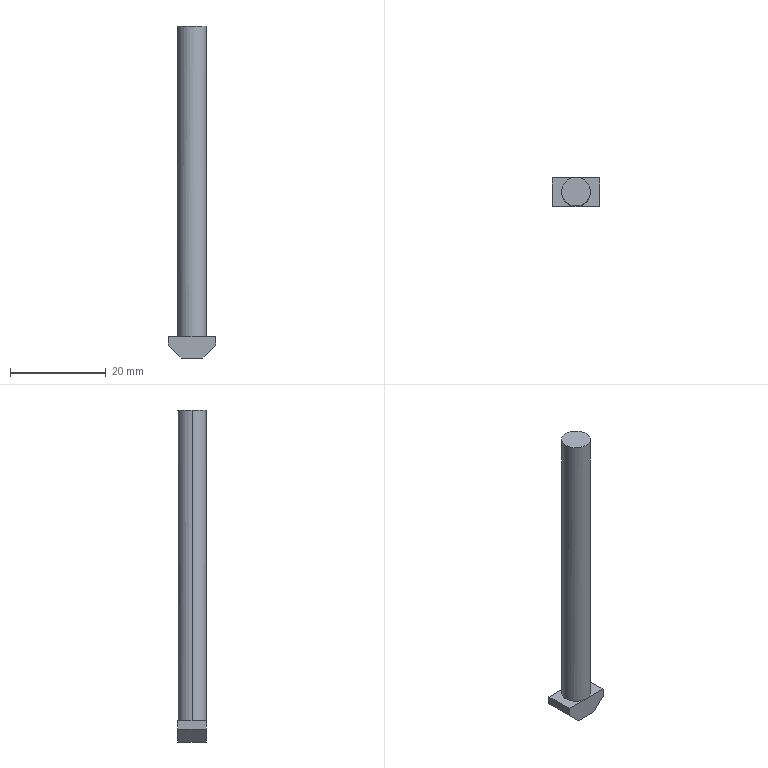Part | SolidWorks | features Extrusion 1, ICE 1 | 1 solid | 12 faces | box 10 x 6 x 69.5 mm | volume 2064 mm3 | plane 10 | cylinder 2 | commonest cylinder face diameters 6 x2
STEP:
#1=CARTESIAN_POINT('',(1.12,3.,52.132));
#2=VERTEX_POINT('',#1);
#3=CARTESIAN_POINT('',(-4.88,3.,52.132));
#4=VERTEX_POINT('',#3);
#5=CARTESIAN_POINT('',(-1.88,3.,52.132));
#6=DIRECTION('',(0.,0.,1.));
#7=DIRECTION('',(1.,0.,0.));
#8=AXIS2_PLACEMENT_3D('',#5,#6,#7);
#9=CIRCLE('',#8,3.);
#10=EDGE_CURVE('',#2,#4,#9,.T.);
#11=ORIENTED_EDGE('',*,*,#10,.F.);
#12=CARTESIAN_POINT('',(1.12,3.,-12.868));
#13=VERTEX_POINT('',#12);
#14=CARTESIAN_POINT('',(1.12,3.,52.132));
#15=DIRECTION('',(0.,0.,-1.));
#16=VECTOR('',#15,1000.);
#17=LINE('',#14,#16);
#18=EDGE_CURVE('',#2,#13,#17,.T.);
#19=ORIENTED_EDGE('',*,*,#18,.T.);
#20=CARTESIAN_POINT('',(-1.88,6.,-12.868));
#21=VERTEX_POINT('',#20);
#22=CARTESIAN_POINT('',(-1.88,3.,-12.868));
#23=DIRECTION('',(0.,0.,1.));
#24=DIRECTION('',(1.,0.,0.));
#25=AXIS2_PLACEMENT_3D('',#22,#23,#24);
#26=CIRCLE('',#25,3.);
#27=EDGE_CURVE('',#13,#21,#26,.T.);
#28=ORIENTED_EDGE('',*,*,#27,.T.);
#29=CARTESIAN_POINT('',(-4.88,3.,-12.868));
#30=VERTEX_POINT('',#29);
#31=CARTESIAN_POINT('',(-1.88,3.,-12.868));
#32=DIRECTION('',(0.,0.,1.));
#33=DIRECTION('',(1.,0.,0.));
#34=AXIS2_PLACEMENT_3D('',#31,#32,#33);
#35=CIRCLE('',#34,3.);
#36=EDGE_CURVE('',#21,#30,#35,.T.);
#37=ORIENTED_EDGE('',*,*,#36,.T.);
#38=CARTESIAN_POINT('',(-4.88,3.,52.132));
#39=DIRECTION('',(0.,0.,-1.));
#40=VECTOR('',#39,1000.);
#41=LINE('',#38,#40);
#42=EDGE_CURVE('',#4,#30,#41,.T.);
#43=ORIENTED_EDGE('',*,*,#42,.F.);
#44=EDGE_LOOP('',(#11,#19,#28,#37,#43));
#45=FACE_OUTER_BOUND('',#44,.T.);
#46=CARTESIAN_POINT('',(-1.88,3.,52.132));
#47=DIRECTION('',(0.,0.,-1.));
#48=DIRECTION('',(-1.,0.,0.));
#49=AXIS2_PLACEMENT_3D('',#46,#47,#48);
#50=CYLINDRICAL_SURFACE('',#49,3.);
#51=ADVANCED_FACE('',(#45),#50,.T.);
#52=ORIENTED_EDGE('',*,*,#36,.F.);
#53=CARTESIAN_POINT('',(-6.88,6.,-12.868));
#54=VERTEX_POINT('',#53);
#55=CARTESIAN_POINT('',(-6.88,6.,-12.868));
#56=DIRECTION('',(1.,0.,0.));
#57=VECTOR('',#56,1000.);
#58=LINE('',#55,#57);
#59=EDGE_CURVE('',#54,#21,#58,.T.);
#60=ORIENTED_EDGE('',*,*,#59,.F.);
#61=CARTESIAN_POINT('',(-6.88,0.,-12.868));
#62=VERTEX_POINT('',#61);
#63=CARTESIAN_POINT('',(-6.88,6.,-12.868));
#64=DIRECTION('',(0.,-1.,0.));
#65=VECTOR('',#64,1000.);
#66=LINE('',#63,#65);
#67=EDGE_CURVE('',#54,#62,#66,.T.);
#68=ORIENTED_EDGE('',*,*,#67,.T.);
#69=CARTESIAN_POINT('',(-1.88,0.,-12.868));
#70=VERTEX_POINT('',#69);
#71=CARTESIAN_POINT('',(-6.88,0.,-12.868));
#72=DIRECTION('',(1.,0.,0.));
#73=VECTOR('',#72,1000.);
#74=LINE('',#71,#73);
#75=EDGE_CURVE('',#62,#70,#74,.T.);
#76=ORIENTED_EDGE('',*,*,#75,.T.);
#77=CARTESIAN_POINT('',(-1.88,3.,-12.868));
#78=DIRECTION('',(0.,0.,1.));
#79=DIRECTION('',(1.,0.,0.));
#80=AXIS2_PLACEMENT_3D('',#77,#78,#79);
#81=CIRCLE('',#80,3.);
#82=EDGE_CURVE('',#30,#70,#81,.T.);
#83=ORIENTED_EDGE('',*,*,#82,.F.);
#84=EDGE_LOOP('',(#52,#60,#68,#76,#83));
#85=FACE_OUTER_BOUND('',#84,.T.);
#86=CARTESIAN_POINT('',(-6.88,6.,-12.868));
#87=DIRECTION('',(0.,0.,-1.));
#88=DIRECTION('',(-1.,0.,0.));
#89=AXIS2_PLACEMENT_3D('',#86,#87,#88);
#90=PLANE('',#89);
#91=ADVANCED_FACE('',(#85),#90,.F.);
#92=CARTESIAN_POINT('',(-6.88,0.,-14.668));
#93=VERTEX_POINT('',#92);
#94=CARTESIAN_POINT('',(-6.88,0.,-12.868));
#95=DIRECTION('',(0.,0.,1.));
#96=VECTOR('',#95,1000.);
#97=LINE('',#94,#96);
#98=EDGE_CURVE('',#93,#62,#97,.T.);
#99=ORIENTED_EDGE('',*,*,#98,.T.);
#100=ORIENTED_EDGE('',*,*,#67,.F.);
#101=CARTESIAN_POINT('',(-6.88,6.,-14.668));
#102=VERTEX_POINT('',#101);
#103=CARTESIAN_POINT('',(-6.88,6.,-12.868));
#104=DIRECTION('',(0.,0.,1.));
#105=VECTOR('',#104,1000.);
#106=LINE('',#103,#105);
#107=EDGE_CURVE('',#102,#54,#106,.T.);
#108=ORIENTED_EDGE('',*,*,#107,.F.);
#109=CARTESIAN_POINT('',(-6.88,6.,-14.668));
#110=DIRECTION('',(0.,-1.,0.));
#111=VECTOR('',#110,1000.);
#112=LINE('',#109,#111);
#113=EDGE_CURVE('',#102,#93,#112,.T.);
#114=ORIENTED_EDGE('',*,*,#113,.T.);
#115=EDGE_LOOP('',(#99,#100,#108,#114));
#116=FACE_OUTER_BOUND('',#115,.T.);
#117=CARTESIAN_POINT('',(-6.88,6.,-12.868));
#118=DIRECTION('',(1.,0.,0.));
#119=DIRECTION('',(0.,0.,-1.));
#120=AXIS2_PLACEMENT_3D('',#117,#118,#119);
#121=PLANE('',#120);
#122=ADVANCED_FACE('',(#116),#121,.F.);
#123=CARTESIAN_POINT('',(-1.88,3.,-12.868));
#124=DIRECTION('',(0.,0.,1.));
#125=DIRECTION('',(1.,0.,0.));
#126=AXIS2_PLACEMENT_3D('',#123,#124,#125);
#127=CIRCLE('',#126,3.);
#128=EDGE_CURVE('',#70,#13,#127,.T.);
#129=ORIENTED_EDGE('',*,*,#128,.F.);
#130=CARTESIAN_POINT('',(3.12,0.,-12.868));
#131=VERTEX_POINT('',#130);
#132=CARTESIAN_POINT('',(-6.88,0.,-12.868));
#133=DIRECTION('',(1.,0.,0.));
#134=VECTOR('',#133,1000.);
#135=LINE('',#132,#134);
#136=EDGE_CURVE('',#70,#131,#135,.T.);
#137=ORIENTED_EDGE('',*,*,#136,.T.);
#138=CARTESIAN_POINT('',(3.12,6.,-12.868));
#139=VERTEX_POINT('',#138);
#140=CARTESIAN_POINT('',(3.12,6.,-12.868));
#141=DIRECTION('',(0.,-1.,0.));
#142=VECTOR('',#141,1000.);
#143=LINE('',#140,#142);
#144=EDGE_CURVE('',#139,#131,#143,.T.);
#145=ORIENTED_EDGE('',*,*,#144,.F.);
#146=CARTESIAN_POINT('',(-6.88,6.,-12.868));
#147=DIRECTION('',(1.,0.,0.));
#148=VECTOR('',#147,1000.);
#149=LINE('',#146,#148);
#150=EDGE_CURVE('',#21,#139,#149,.T.);
#151=ORIENTED_EDGE('',*,*,#150,.F.);
#152=ORIENTED_EDGE('',*,*,#27,.F.);
#153=EDGE_LOOP('',(#129,#137,#145,#151,#152));
#154=FACE_OUTER_BOUND('',#153,.T.);
#155=CARTESIAN_POINT('',(-6.88,6.,-12.868));
#156=DIRECTION('',(0.,0.,-1.));
#157=DIRECTION('',(-1.,0.,0.));
#158=AXIS2_PLACEMENT_3D('',#155,#156,#157);
#159=PLANE('',#158);
#160=ADVANCED_FACE('',(#154),#159,.F.);
#161=CARTESIAN_POINT('',(3.12,0.,-14.668));
#162=VERTEX_POINT('',#161);
#163=CARTESIAN_POINT('',(3.12,0.,-12.868));
#164=DIRECTION('',(0.,0.,-1.));
#165=VECTOR('',#164,1000.);
#166=LINE('',#163,#165);
#167=EDGE_CURVE('',#131,#162,#166,.T.);
#168=ORIENTED_EDGE('',*,*,#167,.T.);
#169=CARTESIAN_POINT('',(3.12,6.,-14.668));
#170=VERTEX_POINT('',#169);
#171=CARTESIAN_POINT('',(3.12,6.,-14.668));
#172=DIRECTION('',(0.,-1.,0.));
#173=VECTOR('',#172,1000.);
#174=LINE('',#171,#173);
#175=EDGE_CURVE('',#170,#162,#174,.T.);
#176=ORIENTED_EDGE('',*,*,#175,.F.);
#177=CARTESIAN_POINT('',(3.12,6.,-12.868));
#178=DIRECTION('',(0.,0.,-1.));
#179=VECTOR('',#178,1000.);
#180=LINE('',#177,#179);
#181=EDGE_CURVE('',#139,#170,#180,.T.);
#182=ORIENTED_EDGE('',*,*,#181,.F.);
#183=ORIENTED_EDGE('',*,*,#144,.T.);
#184=EDGE_LOOP('',(#168,#176,#182,#183));
#185=FACE_OUTER_BOUND('',#184,.T.);
#186=CARTESIAN_POINT('',(3.12,6.,-12.868));
#187=DIRECTION('',(-1.,0.,0.));
#188=DIRECTION('',(0.,0.,1.));
#189=AXIS2_PLACEMENT_3D('',#186,#187,#188);
#190=PLANE('',#189);
#191=ADVANCED_FACE('',(#185),#190,.F.);
#192=CARTESIAN_POINT('',(0.4203,0.,-17.368));
#193=VERTEX_POINT('',#192);
#194=CARTESIAN_POINT('',(3.12,0.,-14.668));
#195=DIRECTION('',(-0.7071,0.,-0.7071));
#196=VECTOR('',#195,1000.);
#197=LINE('',#194,#196);
#198=EDGE_CURVE('',#162,#193,#197,.T.);
#199=ORIENTED_EDGE('',*,*,#198,.T.);
#200=CARTESIAN_POINT('',(0.4203,6.,-17.368));
#201=VERTEX_POINT('',#200);
#202=CARTESIAN_POINT('',(0.4203,6.,-17.368));
#203=DIRECTION('',(0.,-1.,0.));
#204=VECTOR('',#203,1000.);
#205=LINE('',#202,#204);
#206=EDGE_CURVE('',#201,#193,#205,.T.);
#207=ORIENTED_EDGE('',*,*,#206,.F.);
#208=CARTESIAN_POINT('',(3.12,6.,-14.668));
#209=DIRECTION('',(-0.7071,0.,-0.7071));
#210=VECTOR('',#209,1000.);
#211=LINE('',#208,#210);
#212=EDGE_CURVE('',#170,#201,#211,.T.);
#213=ORIENTED_EDGE('',*,*,#212,.F.);
#214=ORIENTED_EDGE('',*,*,#175,.T.);
#215=EDGE_LOOP('',(#199,#207,#213,#214));
#216=FACE_OUTER_BOUND('',#215,.T.);
#217=CARTESIAN_POINT('',(3.12,6.,-14.668));
#218=DIRECTION('',(-0.7071,0.,0.7071));
#219=DIRECTION('',(0.7071,0.,0.7071));
#220=AXIS2_PLACEMENT_3D('',#217,#218,#219);
#221=PLANE('',#220);
#222=ADVANCED_FACE('',(#216),#221,.F.);
#223=CARTESIAN_POINT('',(-4.18,0.,-17.368));
#224=VERTEX_POINT('',#223);
#225=CARTESIAN_POINT('',(0.4203,0.,-17.368));
#226=DIRECTION('',(-1.,0.,0.));
#227=VECTOR('',#226,1000.);
#228=LINE('',#225,#227);
#229=EDGE_CURVE('',#193,#224,#228,.T.);
#230=ORIENTED_EDGE('',*,*,#229,.T.);
#231=CARTESIAN_POINT('',(-4.18,6.,-17.368));
#232=VERTEX_POINT('',#231);
#233=CARTESIAN_POINT('',(-4.18,6.,-17.368));
#234=DIRECTION('',(0.,-1.,0.));
#235=VECTOR('',#234,1000.);
#236=LINE('',#233,#235);
#237=EDGE_CURVE('',#232,#224,#236,.T.);
#238=ORIENTED_EDGE('',*,*,#237,.F.);
#239=CARTESIAN_POINT('',(0.4203,6.,-17.368));
#240=DIRECTION('',(-1.,0.,0.));
#241=VECTOR('',#240,1000.);
#242=LINE('',#239,#241);
#243=EDGE_CURVE('',#201,#232,#242,.T.);
#244=ORIENTED_EDGE('',*,*,#243,.F.);
#245=ORIENTED_EDGE('',*,*,#206,.T.);
#246=EDGE_LOOP('',(#230,#238,#244,#245));
#247=FACE_OUTER_BOUND('',#246,.T.);
#248=CARTESIAN_POINT('',(0.4203,6.,-17.368));
#249=DIRECTION('',(0.,0.,1.));
#250=DIRECTION('',(1.,0.,0.));
#251=AXIS2_PLACEMENT_3D('',#248,#249,#250);
#252=PLANE('',#251);
#253=ADVANCED_FACE('',(#247),#252,.F.);
#254=CARTESIAN_POINT('',(-6.88,0.,-14.668));
#255=DIRECTION('',(-0.7071,0.,0.7071));
#256=VECTOR('',#255,1000.);
#257=LINE('',#254,#256);
#258=EDGE_CURVE('',#224,#93,#257,.T.);
#259=ORIENTED_EDGE('',*,*,#258,.T.);
#260=ORIENTED_EDGE('',*,*,#113,.F.);
#261=CARTESIAN_POINT('',(-6.88,6.,-14.668));
#262=DIRECTION('',(-0.7071,0.,0.7071));
#263=VECTOR('',#262,1000.);
#264=LINE('',#261,#263);
#265=EDGE_CURVE('',#232,#102,#264,.T.);
#266=ORIENTED_EDGE('',*,*,#265,.F.);
#267=ORIENTED_EDGE('',*,*,#237,.T.);
#268=EDGE_LOOP('',(#259,#260,#266,#267));
#269=FACE_OUTER_BOUND('',#268,.T.);
#270=CARTESIAN_POINT('',(-6.88,6.,-14.668));
#271=DIRECTION('',(0.7071,0.,0.7071));
#272=DIRECTION('',(0.7071,0.,-0.7071));
#273=AXIS2_PLACEMENT_3D('',#270,#271,#272);
#274=PLANE('',#273);
#275=ADVANCED_FACE('',(#269),#274,.F.);
#276=ORIENTED_EDGE('',*,*,#107,.T.);
#277=ORIENTED_EDGE('',*,*,#59,.T.);
#278=ORIENTED_EDGE('',*,*,#150,.T.);
#279=ORIENTED_EDGE('',*,*,#181,.T.);
#280=ORIENTED_EDGE('',*,*,#212,.T.);
#281=ORIENTED_EDGE('',*,*,#243,.T.);
#282=ORIENTED_EDGE('',*,*,#265,.T.);
#283=EDGE_LOOP('',(#276,#277,#278,#279,#280,#281,#282));
#284=FACE_OUTER_BOUND('',#283,.T.);
#285=CARTESIAN_POINT('',(0.,6.,0.));
#286=DIRECTION('',(0.,1.,0.));
#287=DIRECTION('',(0.,0.,1.));
#288=AXIS2_PLACEMENT_3D('',#285,#286,#287);
#289=PLANE('',#288);
#290=ADVANCED_FACE('',(#284),#289,.T.);
#291=ORIENTED_EDGE('',*,*,#98,.F.);
#292=ORIENTED_EDGE('',*,*,#258,.F.);
#293=ORIENTED_EDGE('',*,*,#229,.F.);
#294=ORIENTED_EDGE('',*,*,#198,.F.);
#295=ORIENTED_EDGE('',*,*,#167,.F.);
#296=ORIENTED_EDGE('',*,*,#136,.F.);
#297=ORIENTED_EDGE('',*,*,#75,.F.);
#298=EDGE_LOOP('',(#291,#292,#293,#294,#295,#296,#297));
#299=FACE_OUTER_BOUND('',#298,.T.);
#300=CARTESIAN_POINT('',(0.,0.,0.));
#301=DIRECTION('',(0.,1.,0.));
#302=DIRECTION('',(0.,0.,1.));
#303=AXIS2_PLACEMENT_3D('',#300,#301,#302);
#304=PLANE('',#303);
#305=ADVANCED_FACE('',(#299),#304,.F.);
#306=ORIENTED_EDGE('',*,*,#18,.F.);
#307=CARTESIAN_POINT('',(-1.88,3.,52.132));
#308=DIRECTION('',(0.,0.,1.));
#309=DIRECTION('',(1.,0.,0.));
#310=AXIS2_PLACEMENT_3D('',#307,#308,#309);
#311=CIRCLE('',#310,3.);
#312=EDGE_CURVE('',#4,#2,#311,.T.);
#313=ORIENTED_EDGE('',*,*,#312,.F.);
#314=ORIENTED_EDGE('',*,*,#42,.T.);
#315=ORIENTED_EDGE('',*,*,#82,.T.);
#316=ORIENTED_EDGE('',*,*,#128,.T.);
#317=EDGE_LOOP('',(#306,#313,#314,#315,#316));
#318=FACE_OUTER_BOUND('',#317,.T.);
#319=CARTESIAN_POINT('',(-1.88,3.,52.132));
#320=DIRECTION('',(0.,0.,-1.));
#321=DIRECTION('',(-1.,0.,0.));
#322=AXIS2_PLACEMENT_3D('',#319,#320,#321);
#323=CYLINDRICAL_SURFACE('',#322,3.);
#324=ADVANCED_FACE('',(#318),#323,.T.);
#325=ORIENTED_EDGE('',*,*,#312,.T.);
#326=ORIENTED_EDGE('',*,*,#10,.T.);
#327=EDGE_LOOP('',(#325,#326));
#328=FACE_OUTER_BOUND('',#327,.T.);
#329=CARTESIAN_POINT('',(-1.88,3.,52.132));
#330=DIRECTION('',(0.,0.,1.));
#331=DIRECTION('',(1.,0.,0.));
#332=AXIS2_PLACEMENT_3D('',#329,#330,#331);
#333=PLANE('',#332);
#334=ADVANCED_FACE('',(#328),#333,.T.);
#335=CLOSED_SHELL('',(#51,#91,#122,#160,#191,#222,#253,#275,#290,#305,#324,#334));
#336=MANIFOLD_SOLID_BREP('',#335);
#337=CARTESIAN_POINT('',(0.,0.,0.));
#338=DIRECTION('',(0.,0.,1.));
#339=DIRECTION('',(1.,0.,0.));
#340=AXIS2_PLACEMENT_3D('',#337,#338,#339);
#341=(LENGTH_UNIT()NAMED_UNIT(*)SI_UNIT(.MILLI.,.METRE.));
#342=UNCERTAINTY_MEASURE_WITH_UNIT(LENGTH_MEASURE(0.00001),#341,'','');
#343=(NAMED_UNIT(*)PLANE_ANGLE_UNIT()SI_UNIT($,.RADIAN.));
#344=(NAMED_UNIT(*)SI_UNIT($,.STERADIAN.)SOLID_ANGLE_UNIT());
#345=(GEOMETRIC_REPRESENTATION_CONTEXT(3)GLOBAL_UNCERTAINTY_ASSIGNED_CONTEXT((#342))GLOBAL_UNIT_ASSIGNED_CONTEXT((#341,#343,#344))REPRESENTATION_CONTEXT('',''));
#346=ADVANCED_BREP_SHAPE_REPRESENTATION('',(#336,#340),#345);